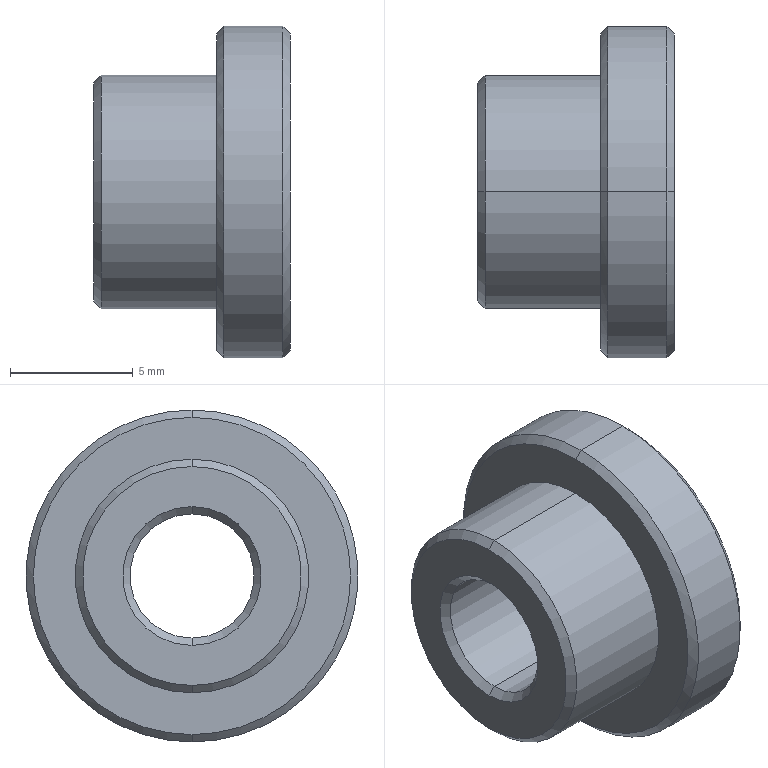Part | STEP file | Transition Guide Wheel | 1 solid | 19 faces | box 8 x 13.5 x 13.5 mm | volume 617.031 mm3 | cone 10 | cylinder 6 | plane 3 | commonest cylinder face diameters 5.05 x2 9.5 x2 13.5 x2
STEP:
#1=CARTESIAN_POINT('',(0.,0.,0.));
#2=DIRECTION('',(0.,0.,1.));
#3=DIRECTION('',(1.,0.,0.));
#4=AXIS2_PLACEMENT_3D('',#1,#2,#3);
#5=CARTESIAN_POINT('',(0.,0.,6.45));
#6=VERTEX_POINT('',#5);
#7=CARTESIAN_POINT('',(0.,0.,-6.45));
#8=VERTEX_POINT('',#7);
#9=CARTESIAN_POINT('',(0.,0.,0.));
#10=DIRECTION('',(-1.,0.,0.));
#11=DIRECTION('',(0.,0.,1.));
#12=AXIS2_PLACEMENT_3D('',#9,#10,#11);
#13=CIRCLE('',#12,6.45);
#14=CARTESIAN_POINT('',(0.3,0.,0.));
#15=DIRECTION('',(1.,0.,0.));
#16=DIRECTION('',(0.,0.,-1.));
#17=AXIS2_PLACEMENT_3D('',#14,#15,#16);
#18=CONICAL_SURFACE('',#17,6.75,0.7854);
#19=CARTESIAN_POINT('',(3.142,-0.3));
#20=DIRECTION('',(-1.,0.));
#21=VECTOR('',#20,1.);
#22=LINE('',#19,#21);
#23=(GEOMETRIC_REPRESENTATION_CONTEXT(2)PARAMETRIC_REPRESENTATION_CONTEXT()REPRESENTATION_CONTEXT('',''));
#24=DEFINITIONAL_REPRESENTATION('',(#22),#23);
#25=PCURVE('',#18,#24);
#26=CARTESIAN_POINT('',(0.,4.75,0.));
#27=DIRECTION('',(-1.,0.,0.));
#28=DIRECTION('',(0.,0.,1.));
#29=AXIS2_PLACEMENT_3D('',#26,#27,#28);
#30=PLANE('',#29);
#31=CARTESIAN_POINT('',(0.,-4.75));
#32=DIRECTION('',(1.,0.));
#33=AXIS2_PLACEMENT_2D('',#31,#32);
#34=CIRCLE('',#33,6.45);
#35=(GEOMETRIC_REPRESENTATION_CONTEXT(2)PARAMETRIC_REPRESENTATION_CONTEXT()REPRESENTATION_CONTEXT('',''));
#36=DEFINITIONAL_REPRESENTATION('',(#34),#35);
#37=PCURVE('',#30,#36);
#38=SURFACE_CURVE('',#13,(#25,#37),.PCURVE_S1.);
#39=EDGE_CURVE('',#6,#8,#38,.T.);
#40=ORIENTED_EDGE('',*,*,#39,.F.);
#41=CARTESIAN_POINT('',(0.3,0.,6.75));
#42=VERTEX_POINT('',#41);
#43=CARTESIAN_POINT('',(0.3,0.,6.75));
#44=DIRECTION('',(0.7071,0.,0.7071));
#45=VECTOR('',#44,1.);
#46=LINE('',#43,#45);
#47=CARTESIAN_POINT('',(3.142,0.));
#48=DIRECTION('',(0.,1.));
#49=VECTOR('',#48,1.);
#50=LINE('',#47,#49);
#51=(GEOMETRIC_REPRESENTATION_CONTEXT(2)PARAMETRIC_REPRESENTATION_CONTEXT()REPRESENTATION_CONTEXT('',''));
#52=DEFINITIONAL_REPRESENTATION('',(#50),#51);
#53=PCURVE('',#18,#52);
#54=CARTESIAN_POINT('',(0.3,0.,0.));
#55=DIRECTION('',(1.,0.,0.));
#56=DIRECTION('',(0.,0.,-1.));
#57=AXIS2_PLACEMENT_3D('',#54,#55,#56);
#58=CONICAL_SURFACE('',#57,6.75,0.7854);
#59=CARTESIAN_POINT('',(3.142,0.));
#60=DIRECTION('',(0.,1.));
#61=VECTOR('',#60,1.);
#62=LINE('',#59,#61);
#63=(GEOMETRIC_REPRESENTATION_CONTEXT(2)PARAMETRIC_REPRESENTATION_CONTEXT()REPRESENTATION_CONTEXT('',''));
#64=DEFINITIONAL_REPRESENTATION('',(#62),#63);
#65=PCURVE('',#58,#64);
#66=SURFACE_CURVE('',#46,(#53,#65),.PCURVE_S1.);
#67=EDGE_CURVE('',#6,#42,#66,.T.);
#68=ORIENTED_EDGE('',*,*,#67,.T.);
#69=CARTESIAN_POINT('',(0.3,0.,-6.75));
#70=VERTEX_POINT('',#69);
#71=CARTESIAN_POINT('',(0.3,0.,0.));
#72=DIRECTION('',(1.,0.,0.));
#73=DIRECTION('',(0.,0.,1.));
#74=AXIS2_PLACEMENT_3D('',#71,#72,#73);
#75=CIRCLE('',#74,6.75);
#76=CARTESIAN_POINT('',(-3.142,0.));
#77=DIRECTION('',(1.,0.));
#78=VECTOR('',#77,1.);
#79=LINE('',#76,#78);
#80=(GEOMETRIC_REPRESENTATION_CONTEXT(2)PARAMETRIC_REPRESENTATION_CONTEXT()REPRESENTATION_CONTEXT('',''));
#81=DEFINITIONAL_REPRESENTATION('',(#79),#80);
#82=PCURVE('',#18,#81);
#83=CARTESIAN_POINT('',(0.,0.,0.));
#84=DIRECTION('',(1.,0.,0.));
#85=DIRECTION('',(0.,0.,-1.));
#86=AXIS2_PLACEMENT_3D('',#83,#84,#85);
#87=CYLINDRICAL_SURFACE('',#86,6.75);
#88=CARTESIAN_POINT('',(-3.142,0.3));
#89=DIRECTION('',(1.,0.));
#90=VECTOR('',#89,1.);
#91=LINE('',#88,#90);
#92=(GEOMETRIC_REPRESENTATION_CONTEXT(2)PARAMETRIC_REPRESENTATION_CONTEXT()REPRESENTATION_CONTEXT('',''));
#93=DEFINITIONAL_REPRESENTATION('',(#91),#92);
#94=PCURVE('',#87,#93);
#95=SURFACE_CURVE('',#75,(#82,#94),.PCURVE_S1.);
#96=EDGE_CURVE('',#70,#42,#95,.T.);
#97=ORIENTED_EDGE('',*,*,#96,.F.);
#98=CARTESIAN_POINT('',(0.3,0.,-6.75));
#99=DIRECTION('',(0.7071,0.,-0.7071));
#100=VECTOR('',#99,1.);
#101=LINE('',#98,#100);
#102=CARTESIAN_POINT('',(0.,0.));
#103=DIRECTION('',(0.,1.));
#104=VECTOR('',#103,1.);
#105=LINE('',#102,#104);
#106=(GEOMETRIC_REPRESENTATION_CONTEXT(2)PARAMETRIC_REPRESENTATION_CONTEXT()REPRESENTATION_CONTEXT('',''));
#107=DEFINITIONAL_REPRESENTATION('',(#105),#106);
#108=PCURVE('',#18,#107);
#109=CARTESIAN_POINT('',(6.283,0.));
#110=DIRECTION('',(0.,1.));
#111=VECTOR('',#110,1.);
#112=LINE('',#109,#111);
#113=(GEOMETRIC_REPRESENTATION_CONTEXT(2)PARAMETRIC_REPRESENTATION_CONTEXT()REPRESENTATION_CONTEXT('',''));
#114=DEFINITIONAL_REPRESENTATION('',(#112),#113);
#115=PCURVE('',#58,#114);
#116=SURFACE_CURVE('',#101,(#108,#115),.PCURVE_S1.);
#117=EDGE_CURVE('',#8,#70,#116,.T.);
#118=ORIENTED_EDGE('',*,*,#117,.F.);
#119=EDGE_LOOP('',(#40,#68,#97,#118));
#120=FACE_BOUND('',#119,.T.);
#121=ADVANCED_FACE('',(#120),#18,.T.);
#122=CARTESIAN_POINT('',(3.,0.,-6.45));
#123=VERTEX_POINT('',#122);
#124=CARTESIAN_POINT('',(3.,0.,6.45));
#125=VERTEX_POINT('',#124);
#126=CARTESIAN_POINT('',(3.,0.,0.));
#127=DIRECTION('',(1.,0.,0.));
#128=DIRECTION('',(0.,0.,-1.));
#129=AXIS2_PLACEMENT_3D('',#126,#127,#128);
#130=CIRCLE('',#129,6.45);
#131=CARTESIAN_POINT('',(3.,0.,0.));
#132=DIRECTION('',(-1.,0.,0.));
#133=DIRECTION('',(0.,0.,1.));
#134=AXIS2_PLACEMENT_3D('',#131,#132,#133);
#135=CONICAL_SURFACE('',#134,6.45,0.7854);
#136=CARTESIAN_POINT('',(3.142,0.));
#137=DIRECTION('',(-1.,0.));
#138=VECTOR('',#137,1.);
#139=LINE('',#136,#138);
#140=(GEOMETRIC_REPRESENTATION_CONTEXT(2)PARAMETRIC_REPRESENTATION_CONTEXT()REPRESENTATION_CONTEXT('',''));
#141=DEFINITIONAL_REPRESENTATION('',(#139),#140);
#142=PCURVE('',#135,#141);
#143=CARTESIAN_POINT('',(3.,6.75,0.));
#144=DIRECTION('',(1.,0.,0.));
#145=DIRECTION('',(0.,0.,-1.));
#146=AXIS2_PLACEMENT_3D('',#143,#144,#145);
#147=PLANE('',#146);
#148=CARTESIAN_POINT('',(0.,-6.75));
#149=DIRECTION('',(1.,0.));
#150=AXIS2_PLACEMENT_2D('',#148,#149);
#151=CIRCLE('',#150,6.45);
#152=(GEOMETRIC_REPRESENTATION_CONTEXT(2)PARAMETRIC_REPRESENTATION_CONTEXT()REPRESENTATION_CONTEXT('',''));
#153=DEFINITIONAL_REPRESENTATION('',(#151),#152);
#154=PCURVE('',#147,#153);
#155=SURFACE_CURVE('',#130,(#142,#154),.PCURVE_S1.);
#156=EDGE_CURVE('',#123,#125,#155,.T.);
#157=ORIENTED_EDGE('',*,*,#156,.F.);
#158=CARTESIAN_POINT('',(2.7,0.,-6.75));
#159=VERTEX_POINT('',#158);
#160=CARTESIAN_POINT('',(3.,0.,-6.45));
#161=DIRECTION('',(-0.7071,0.,-0.7071));
#162=VECTOR('',#161,1.);
#163=LINE('',#160,#162);
#164=CARTESIAN_POINT('',(3.142,0.));
#165=DIRECTION('',(0.,1.));
#166=VECTOR('',#165,1.);
#167=LINE('',#164,#166);
#168=(GEOMETRIC_REPRESENTATION_CONTEXT(2)PARAMETRIC_REPRESENTATION_CONTEXT()REPRESENTATION_CONTEXT('',''));
#169=DEFINITIONAL_REPRESENTATION('',(#167),#168);
#170=PCURVE('',#135,#169);
#171=CARTESIAN_POINT('',(3.,0.,0.));
#172=DIRECTION('',(-1.,0.,0.));
#173=DIRECTION('',(0.,0.,1.));
#174=AXIS2_PLACEMENT_3D('',#171,#172,#173);
#175=CONICAL_SURFACE('',#174,6.45,0.7854);
#176=CARTESIAN_POINT('',(3.142,0.));
#177=DIRECTION('',(0.,1.));
#178=VECTOR('',#177,1.);
#179=LINE('',#176,#178);
#180=(GEOMETRIC_REPRESENTATION_CONTEXT(2)PARAMETRIC_REPRESENTATION_CONTEXT()REPRESENTATION_CONTEXT('',''));
#181=DEFINITIONAL_REPRESENTATION('',(#179),#180);
#182=PCURVE('',#175,#181);
#183=SURFACE_CURVE('',#163,(#170,#182),.PCURVE_S1.);
#184=EDGE_CURVE('',#123,#159,#183,.T.);
#185=ORIENTED_EDGE('',*,*,#184,.T.);
#186=CARTESIAN_POINT('',(2.7,0.,6.75));
#187=VERTEX_POINT('',#186);
#188=CARTESIAN_POINT('',(2.7,0.,0.));
#189=DIRECTION('',(-1.,0.,0.));
#190=DIRECTION('',(0.,0.,-1.));
#191=AXIS2_PLACEMENT_3D('',#188,#189,#190);
#192=CIRCLE('',#191,6.75);
#193=CARTESIAN_POINT('',(-3.142,0.3));
#194=DIRECTION('',(1.,0.));
#195=VECTOR('',#194,1.);
#196=LINE('',#193,#195);
#197=(GEOMETRIC_REPRESENTATION_CONTEXT(2)PARAMETRIC_REPRESENTATION_CONTEXT()REPRESENTATION_CONTEXT('',''));
#198=DEFINITIONAL_REPRESENTATION('',(#196),#197);
#199=PCURVE('',#135,#198);
#200=CARTESIAN_POINT('',(6.283,2.7));
#201=DIRECTION('',(-1.,0.));
#202=VECTOR('',#201,1.);
#203=LINE('',#200,#202);
#204=(GEOMETRIC_REPRESENTATION_CONTEXT(2)PARAMETRIC_REPRESENTATION_CONTEXT()REPRESENTATION_CONTEXT('',''));
#205=DEFINITIONAL_REPRESENTATION('',(#203),#204);
#206=PCURVE('',#87,#205);
#207=SURFACE_CURVE('',#192,(#199,#206),.PCURVE_S1.);
#208=EDGE_CURVE('',#187,#159,#207,.T.);
#209=ORIENTED_EDGE('',*,*,#208,.F.);
#210=CARTESIAN_POINT('',(3.,0.,6.45));
#211=DIRECTION('',(-0.7071,0.,0.7071));
#212=VECTOR('',#211,1.);
#213=LINE('',#210,#212);
#214=CARTESIAN_POINT('',(0.,0.));
#215=DIRECTION('',(0.,1.));
#216=VECTOR('',#215,1.);
#217=LINE('',#214,#216);
#218=(GEOMETRIC_REPRESENTATION_CONTEXT(2)PARAMETRIC_REPRESENTATION_CONTEXT()REPRESENTATION_CONTEXT('',''));
#219=DEFINITIONAL_REPRESENTATION('',(#217),#218);
#220=PCURVE('',#135,#219);
#221=CARTESIAN_POINT('',(6.283,0.));
#222=DIRECTION('',(0.,1.));
#223=VECTOR('',#222,1.);
#224=LINE('',#221,#223);
#225=(GEOMETRIC_REPRESENTATION_CONTEXT(2)PARAMETRIC_REPRESENTATION_CONTEXT()REPRESENTATION_CONTEXT('',''));
#226=DEFINITIONAL_REPRESENTATION('',(#224),#225);
#227=PCURVE('',#175,#226);
#228=SURFACE_CURVE('',#213,(#220,#227),.PCURVE_S1.);
#229=EDGE_CURVE('',#125,#187,#228,.T.);
#230=ORIENTED_EDGE('',*,*,#229,.F.);
#231=EDGE_LOOP('',(#157,#185,#209,#230));
#232=FACE_BOUND('',#231,.T.);
#233=ADVANCED_FACE('',(#232),#135,.T.);
#234=CARTESIAN_POINT('',(2.7,0.,-2.525));
#235=VERTEX_POINT('',#234);
#236=CARTESIAN_POINT('',(3.,0.,-2.825));
#237=VERTEX_POINT('',#236);
#238=CARTESIAN_POINT('',(2.7,0.,-2.525));
#239=DIRECTION('',(0.7071,0.,-0.7071));
#240=VECTOR('',#239,1.);
#241=LINE('',#238,#240);
#242=CARTESIAN_POINT('',(2.7,0.,0.));
#243=DIRECTION('',(1.,0.,0.));
#244=DIRECTION('',(0.,0.,-1.));
#245=AXIS2_PLACEMENT_3D('',#242,#243,#244);
#246=CONICAL_SURFACE('',#245,2.525,0.7854);
#247=CARTESIAN_POINT('',(6.283,0.));
#248=DIRECTION('',(0.,1.));
#249=VECTOR('',#248,1.);
#250=LINE('',#247,#249);
#251=(GEOMETRIC_REPRESENTATION_CONTEXT(2)PARAMETRIC_REPRESENTATION_CONTEXT()REPRESENTATION_CONTEXT('',''));
#252=DEFINITIONAL_REPRESENTATION('',(#250),#251);
#253=PCURVE('',#246,#252);
#254=CARTESIAN_POINT('',(2.7,0.,0.));
#255=DIRECTION('',(1.,0.,0.));
#256=DIRECTION('',(0.,0.,-1.));
#257=AXIS2_PLACEMENT_3D('',#254,#255,#256);
#258=CONICAL_SURFACE('',#257,2.525,0.7854);
#259=CARTESIAN_POINT('',(0.,0.));
#260=DIRECTION('',(0.,1.));
#261=VECTOR('',#260,1.);
#262=LINE('',#259,#261);
#263=(GEOMETRIC_REPRESENTATION_CONTEXT(2)PARAMETRIC_REPRESENTATION_CONTEXT()REPRESENTATION_CONTEXT('',''));
#264=DEFINITIONAL_REPRESENTATION('',(#262),#263);
#265=PCURVE('',#258,#264);
#266=SURFACE_CURVE('',#241,(#253,#265),.PCURVE_S1.);
#267=EDGE_CURVE('',#235,#237,#266,.T.);
#268=ORIENTED_EDGE('',*,*,#267,.T.);
#269=CARTESIAN_POINT('',(3.,0.,2.825));
#270=VERTEX_POINT('',#269);
#271=CARTESIAN_POINT('',(3.,0.,0.));
#272=DIRECTION('',(-1.,0.,0.));
#273=DIRECTION('',(0.,0.,-1.));
#274=AXIS2_PLACEMENT_3D('',#271,#272,#273);
#275=CIRCLE('',#274,2.825);
#276=CARTESIAN_POINT('',(6.283,0.3));
#277=DIRECTION('',(-1.,0.));
#278=VECTOR('',#277,1.);
#279=LINE('',#276,#278);
#280=(GEOMETRIC_REPRESENTATION_CONTEXT(2)PARAMETRIC_REPRESENTATION_CONTEXT()REPRESENTATION_CONTEXT('',''));
#281=DEFINITIONAL_REPRESENTATION('',(#279),#280);
#282=PCURVE('',#246,#281);
#283=CARTESIAN_POINT('',(2.825,-6.75));
#284=CARTESIAN_POINT('',(2.825,-11.643));
#285=CARTESIAN_POINT('',(-1.413,-9.197));
#286=CARTESIAN_POINT('',(-5.65,-6.75));
#287=CARTESIAN_POINT('',(-1.413,-4.303));
#288=CARTESIAN_POINT('',(2.825,-1.857));
#289=CARTESIAN_POINT('',(2.825,-6.75));
#290=(BOUNDED_CURVE()B_SPLINE_CURVE(2,(#283,#284,#285,#286,#287,#288,#289),.UNSPECIFIED.,.T.,.F.)B_SPLINE_CURVE_WITH_KNOTS((1,2,2,2,2,1),(-2.094,0.,2.094,4.189,6.283,8.378),.UNSPECIFIED.)CURVE()GEOMETRIC_REPRESENTATION_ITEM()RATIONAL_B_SPLINE_CURVE((1.,0.5,1.,0.5,1.,0.5,1.))REPRESENTATION_ITEM(''));
#291=(GEOMETRIC_REPRESENTATION_CONTEXT(2)PARAMETRIC_REPRESENTATION_CONTEXT()REPRESENTATION_CONTEXT('',''));
#292=DEFINITIONAL_REPRESENTATION('',(#290),#291);
#293=PCURVE('',#147,#292);
#294=SURFACE_CURVE('',#275,(#282,#293),.PCURVE_S1.);
#295=EDGE_CURVE('',#237,#270,#294,.T.);
#296=ORIENTED_EDGE('',*,*,#295,.T.);
#297=CARTESIAN_POINT('',(2.7,0.,2.525));
#298=VERTEX_POINT('',#297);
#299=CARTESIAN_POINT('',(2.7,0.,2.525));
#300=DIRECTION('',(0.7071,0.,0.7071));
#301=VECTOR('',#300,1.);
#302=LINE('',#299,#301);
#303=CARTESIAN_POINT('',(3.142,0.));
#304=DIRECTION('',(0.,1.));
#305=VECTOR('',#304,1.);
#306=LINE('',#303,#305);
#307=(GEOMETRIC_REPRESENTATION_CONTEXT(2)PARAMETRIC_REPRESENTATION_CONTEXT()REPRESENTATION_CONTEXT('',''));
#308=DEFINITIONAL_REPRESENTATION('',(#306),#307);
#309=PCURVE('',#246,#308);
#310=CARTESIAN_POINT('',(3.142,0.));
#311=DIRECTION('',(0.,1.));
#312=VECTOR('',#311,1.);
#313=LINE('',#310,#312);
#314=(GEOMETRIC_REPRESENTATION_CONTEXT(2)PARAMETRIC_REPRESENTATION_CONTEXT()REPRESENTATION_CONTEXT('',''));
#315=DEFINITIONAL_REPRESENTATION('',(#313),#314);
#316=PCURVE('',#258,#315);
#317=SURFACE_CURVE('',#302,(#309,#316),.PCURVE_S1.);
#318=EDGE_CURVE('',#298,#270,#317,.T.);
#319=ORIENTED_EDGE('',*,*,#318,.F.);
#320=CARTESIAN_POINT('',(2.7,0.,0.));
#321=DIRECTION('',(1.,0.,0.));
#322=DIRECTION('',(0.,0.,-1.));
#323=AXIS2_PLACEMENT_3D('',#320,#321,#322);
#324=CIRCLE('',#323,2.525);
#325=CARTESIAN_POINT('',(0.,0.));
#326=DIRECTION('',(1.,0.));
#327=VECTOR('',#326,1.);
#328=LINE('',#325,#327);
#329=(GEOMETRIC_REPRESENTATION_CONTEXT(2)PARAMETRIC_REPRESENTATION_CONTEXT()REPRESENTATION_CONTEXT('',''));
#330=DEFINITIONAL_REPRESENTATION('',(#328),#329);
#331=PCURVE('',#246,#330);
#332=CARTESIAN_POINT('',(0.,0.,0.));
#333=DIRECTION('',(1.,0.,0.));
#334=DIRECTION('',(0.,0.,-1.));
#335=AXIS2_PLACEMENT_3D('',#332,#333,#334);
#336=CYLINDRICAL_SURFACE('',#335,2.525);
#337=CARTESIAN_POINT('',(0.,2.7));
#338=DIRECTION('',(1.,0.));
#339=VECTOR('',#338,1.);
#340=LINE('',#337,#339);
#341=(GEOMETRIC_REPRESENTATION_CONTEXT(2)PARAMETRIC_REPRESENTATION_CONTEXT()REPRESENTATION_CONTEXT('',''));
#342=DEFINITIONAL_REPRESENTATION('',(#340),#341);
#343=PCURVE('',#336,#342);
#344=SURFACE_CURVE('',#324,(#331,#343),.PCURVE_S1.);
#345=EDGE_CURVE('',#298,#235,#344,.T.);
#346=ORIENTED_EDGE('',*,*,#345,.T.);
#347=EDGE_LOOP('',(#268,#296,#319,#346));
#348=FACE_BOUND('',#347,.F.);
#349=ADVANCED_FACE('',(#348),#246,.F.);
#350=CARTESIAN_POINT('',(-4.7,0.,2.525));
#351=VERTEX_POINT('',#350);
#352=CARTESIAN_POINT('',(-5.,0.,2.825));
#353=VERTEX_POINT('',#352);
#354=CARTESIAN_POINT('',(-5.,0.,2.825));
#355=DIRECTION('',(-0.7071,0.,0.7071));
#356=VECTOR('',#355,1.);
#357=LINE('',#354,#356);
#358=CARTESIAN_POINT('',(-5.,0.,0.));
#359=DIRECTION('',(-1.,0.,0.));
#360=DIRECTION('',(0.,0.,1.));
#361=AXIS2_PLACEMENT_3D('',#358,#359,#360);
#362=CONICAL_SURFACE('',#361,2.825,0.7854);
#363=CARTESIAN_POINT('',(6.283,0.));
#364=DIRECTION('',(0.,1.));
#365=VECTOR('',#364,1.);
#366=LINE('',#363,#365);
#367=(GEOMETRIC_REPRESENTATION_CONTEXT(2)PARAMETRIC_REPRESENTATION_CONTEXT()REPRESENTATION_CONTEXT('',''));
#368=DEFINITIONAL_REPRESENTATION('',(#366),#367);
#369=PCURVE('',#362,#368);
#370=CARTESIAN_POINT('',(-5.,0.,0.));
#371=DIRECTION('',(-1.,0.,0.));
#372=DIRECTION('',(0.,0.,1.));
#373=AXIS2_PLACEMENT_3D('',#370,#371,#372);
#374=CONICAL_SURFACE('',#373,2.825,0.7854);
#375=CARTESIAN_POINT('',(0.,0.));
#376=DIRECTION('',(0.,1.));
#377=VECTOR('',#376,1.);
#378=LINE('',#375,#377);
#379=(GEOMETRIC_REPRESENTATION_CONTEXT(2)PARAMETRIC_REPRESENTATION_CONTEXT()REPRESENTATION_CONTEXT('',''));
#380=DEFINITIONAL_REPRESENTATION('',(#378),#379);
#381=PCURVE('',#374,#380);
#382=SURFACE_CURVE('',#357,(#369,#381),.PCURVE_S1.);
#383=EDGE_CURVE('',#351,#353,#382,.T.);
#384=ORIENTED_EDGE('',*,*,#383,.T.);
#385=CARTESIAN_POINT('',(-5.,0.,-2.825));
#386=VERTEX_POINT('',#385);
#387=CARTESIAN_POINT('',(-5.,0.,0.));
#388=DIRECTION('',(1.,0.,0.));
#389=DIRECTION('',(0.,0.,1.));
#390=AXIS2_PLACEMENT_3D('',#387,#388,#389);
#391=CIRCLE('',#390,2.825);
#392=CARTESIAN_POINT('',(6.283,0.));
#393=DIRECTION('',(-1.,0.));
#394=VECTOR('',#393,1.);
#395=LINE('',#392,#394);
#396=(GEOMETRIC_REPRESENTATION_CONTEXT(2)PARAMETRIC_REPRESENTATION_CONTEXT()REPRESENTATION_CONTEXT('',''));
#397=DEFINITIONAL_REPRESENTATION('',(#395),#396);
#398=PCURVE('',#362,#397);
#399=CARTESIAN_POINT('',(-5.,2.525,0.));
#400=DIRECTION('',(-1.,0.,0.));
#401=DIRECTION('',(0.,0.,1.));
#402=AXIS2_PLACEMENT_3D('',#399,#400,#401);
#403=PLANE('',#402);
#404=CARTESIAN_POINT('',(2.825,-2.525));
#405=CARTESIAN_POINT('',(2.825,-7.418));
#406=CARTESIAN_POINT('',(-1.413,-4.972));
#407=CARTESIAN_POINT('',(-5.65,-2.525));
#408=CARTESIAN_POINT('',(-1.413,-0.07848));
#409=CARTESIAN_POINT('',(2.825,2.368));
#410=CARTESIAN_POINT('',(2.825,-2.525));
#411=(BOUNDED_CURVE()B_SPLINE_CURVE(2,(#404,#405,#406,#407,#408,#409,#410),.UNSPECIFIED.,.T.,.F.)B_SPLINE_CURVE_WITH_KNOTS((1,2,2,2,2,1),(-2.094,0.,2.094,4.189,6.283,8.378),.UNSPECIFIED.)CURVE()GEOMETRIC_REPRESENTATION_ITEM()RATIONAL_B_SPLINE_CURVE((1.,0.5,1.,0.5,1.,0.5,1.))REPRESENTATION_ITEM(''));
#412=(GEOMETRIC_REPRESENTATION_CONTEXT(2)PARAMETRIC_REPRESENTATION_CONTEXT()REPRESENTATION_CONTEXT('',''));
#413=DEFINITIONAL_REPRESENTATION('',(#411),#412);
#414=PCURVE('',#403,#413);
#415=SURFACE_CURVE('',#391,(#398,#414),.PCURVE_S1.);
#416=EDGE_CURVE('',#353,#386,#415,.T.);
#417=ORIENTED_EDGE('',*,*,#416,.T.);
#418=CARTESIAN_POINT('',(-4.7,0.,-2.525));
#419=VERTEX_POINT('',#418);
#420=CARTESIAN_POINT('',(-5.,0.,-2.825));
#421=DIRECTION('',(-0.7071,0.,-0.7071));
#422=VECTOR('',#421,1.);
#423=LINE('',#420,#422);
#424=CARTESIAN_POINT('',(3.142,0.));
#425=DIRECTION('',(0.,1.));
#426=VECTOR('',#425,1.);
#427=LINE('',#424,#426);
#428=(GEOMETRIC_REPRESENTATION_CONTEXT(2)PARAMETRIC_REPRESENTATION_CONTEXT()REPRESENTATION_CONTEXT('',''));
#429=DEFINITIONAL_REPRESENTATION('',(#427),#428);
#430=PCURVE('',#362,#429);
#431=CARTESIAN_POINT('',(3.142,0.));
#432=DIRECTION('',(0.,1.));
#433=VECTOR('',#432,1.);
#434=LINE('',#431,#433);
#435=(GEOMETRIC_REPRESENTATION_CONTEXT(2)PARAMETRIC_REPRESENTATION_CONTEXT()REPRESENTATION_CONTEXT('',''));
#436=DEFINITIONAL_REPRESENTATION('',(#434),#435);
#437=PCURVE('',#374,#436);
#438=SURFACE_CURVE('',#423,(#430,#437),.PCURVE_S1.);
#439=EDGE_CURVE('',#419,#386,#438,.T.);
#440=ORIENTED_EDGE('',*,*,#439,.F.);
#441=CARTESIAN_POINT('',(-4.7,0.,0.));
#442=DIRECTION('',(-1.,0.,0.));
#443=DIRECTION('',(0.,0.,1.));
#444=AXIS2_PLACEMENT_3D('',#441,#442,#443);
#445=CIRCLE('',#444,2.525);
#446=CARTESIAN_POINT('',(0.,-0.3));
#447=DIRECTION('',(1.,0.));
#448=VECTOR('',#447,1.);
#449=LINE('',#446,#448);
#450=(GEOMETRIC_REPRESENTATION_CONTEXT(2)PARAMETRIC_REPRESENTATION_CONTEXT()REPRESENTATION_CONTEXT('',''));
#451=DEFINITIONAL_REPRESENTATION('',(#449),#450);
#452=PCURVE('',#362,#451);
#453=CARTESIAN_POINT('',(9.425,-4.7));
#454=DIRECTION('',(-1.,0.));
#455=VECTOR('',#454,1.);
#456=LINE('',#453,#455);
#457=(GEOMETRIC_REPRESENTATION_CONTEXT(2)PARAMETRIC_REPRESENTATION_CONTEXT()REPRESENTATION_CONTEXT('',''));
#458=DEFINITIONAL_REPRESENTATION('',(#456),#457);
#459=PCURVE('',#336,#458);
#460=SURFACE_CURVE('',#445,(#452,#459),.PCURVE_S1.);
#461=EDGE_CURVE('',#419,#351,#460,.T.);
#462=ORIENTED_EDGE('',*,*,#461,.T.);
#463=EDGE_LOOP('',(#384,#417,#440,#462));
#464=FACE_BOUND('',#463,.F.);
#465=ADVANCED_FACE('',(#464),#362,.F.);
#466=CARTESIAN_POINT('',(-5.,0.,4.45));
#467=VERTEX_POINT('',#466);
#468=CARTESIAN_POINT('',(-5.,0.,-4.45));
#469=VERTEX_POINT('',#468);
#470=CARTESIAN_POINT('',(-5.,0.,0.));
#471=DIRECTION('',(-1.,0.,0.));
#472=DIRECTION('',(0.,0.,1.));
#473=AXIS2_PLACEMENT_3D('',#470,#471,#472);
#474=CIRCLE('',#473,4.45);
#475=CARTESIAN_POINT('',(-4.7,0.,0.));
#476=DIRECTION('',(1.,0.,0.));
#477=DIRECTION('',(0.,0.,-1.));
#478=AXIS2_PLACEMENT_3D('',#475,#476,#477);
#479=CONICAL_SURFACE('',#478,4.75,0.7854);
#480=CARTESIAN_POINT('',(3.142,-0.3));
#481=DIRECTION('',(-1.,0.));
#482=VECTOR('',#481,1.);
#483=LINE('',#480,#482);
#484=(GEOMETRIC_REPRESENTATION_CONTEXT(2)PARAMETRIC_REPRESENTATION_CONTEXT()REPRESENTATION_CONTEXT('',''));
#485=DEFINITIONAL_REPRESENTATION('',(#483),#484);
#486=PCURVE('',#479,#485);
#487=CARTESIAN_POINT('',(0.,-2.525));
#488=DIRECTION('',(1.,0.));
#489=AXIS2_PLACEMENT_2D('',#487,#488);
#490=CIRCLE('',#489,4.45);
#491=(GEOMETRIC_REPRESENTATION_CONTEXT(2)PARAMETRIC_REPRESENTATION_CONTEXT()REPRESENTATION_CONTEXT('',''));
#492=DEFINITIONAL_REPRESENTATION('',(#490),#491);
#493=PCURVE('',#403,#492);
#494=SURFACE_CURVE('',#474,(#486,#493),.PCURVE_S1.);
#495=EDGE_CURVE('',#467,#469,#494,.T.);
#496=ORIENTED_EDGE('',*,*,#495,.F.);
#497=CARTESIAN_POINT('',(-4.7,0.,4.75));
#498=VERTEX_POINT('',#497);
#499=CARTESIAN_POINT('',(-4.7,0.,4.75));
#500=DIRECTION('',(0.7071,0.,0.7071));
#501=VECTOR('',#500,1.);
#502=LINE('',#499,#501);
#503=CARTESIAN_POINT('',(3.142,0.));
#504=DIRECTION('',(0.,1.));
#505=VECTOR('',#504,1.);
#506=LINE('',#503,#505);
#507=(GEOMETRIC_REPRESENTATION_CONTEXT(2)PARAMETRIC_REPRESENTATION_CONTEXT()REPRESENTATION_CONTEXT('',''));
#508=DEFINITIONAL_REPRESENTATION('',(#506),#507);
#509=PCURVE('',#479,#508);
#510=CARTESIAN_POINT('',(-4.7,0.,0.));
#511=DIRECTION('',(1.,0.,0.));
#512=DIRECTION('',(0.,0.,-1.));
#513=AXIS2_PLACEMENT_3D('',#510,#511,#512);
#514=CONICAL_SURFACE('',#513,4.75,0.7854);
#515=CARTESIAN_POINT('',(3.142,0.));
#516=DIRECTION('',(0.,1.));
#517=VECTOR('',#516,1.);
#518=LINE('',#515,#517);
#519=(GEOMETRIC_REPRESENTATION_CONTEXT(2)PARAMETRIC_REPRESENTATION_CONTEXT()REPRESENTATION_CONTEXT('',''));
#520=DEFINITIONAL_REPRESENTATION('',(#518),#519);
#521=PCURVE('',#514,#520);
#522=SURFACE_CURVE('',#502,(#509,#521),.PCURVE_S1.);
#523=EDGE_CURVE('',#467,#498,#522,.T.);
#524=ORIENTED_EDGE('',*,*,#523,.T.);
#525=CARTESIAN_POINT('',(-4.7,0.,-4.75));
#526=VERTEX_POINT('',#525);
#527=CARTESIAN_POINT('',(-4.7,0.,0.));
#528=DIRECTION('',(1.,0.,0.));
#529=DIRECTION('',(0.,0.,1.));
#530=AXIS2_PLACEMENT_3D('',#527,#528,#529);
#531=CIRCLE('',#530,4.75);
#532=CARTESIAN_POINT('',(-3.142,0.));
#533=DIRECTION('',(1.,0.));
#534=VECTOR('',#533,1.);
#535=LINE('',#532,#534);
#536=(GEOMETRIC_REPRESENTATION_CONTEXT(2)PARAMETRIC_REPRESENTATION_CONTEXT()REPRESENTATION_CONTEXT('',''));
#537=DEFINITIONAL_REPRESENTATION('',(#535),#536);
#538=PCURVE('',#479,#537);
#539=CARTESIAN_POINT('',(0.,0.,0.));
#540=DIRECTION('',(1.,0.,0.));
#541=DIRECTION('',(0.,0.,-1.));
#542=AXIS2_PLACEMENT_3D('',#539,#540,#541);
#543=CYLINDRICAL_SURFACE('',#542,4.75);
#544=CARTESIAN_POINT('',(-3.142,-4.7));
#545=DIRECTION('',(1.,0.));
#546=VECTOR('',#545,1.);
#547=LINE('',#544,#546);
#548=(GEOMETRIC_REPRESENTATION_CONTEXT(2)PARAMETRIC_REPRESENTATION_CONTEXT()REPRESENTATION_CONTEXT('',''));
#549=DEFINITIONAL_REPRESENTATION('',(#547),#548);
#550=PCURVE('',#543,#549);
#551=SURFACE_CURVE('',#531,(#538,#550),.PCURVE_S1.);
#552=EDGE_CURVE('',#526,#498,#551,.T.);
#553=ORIENTED_EDGE('',*,*,#552,.F.);
#554=CARTESIAN_POINT('',(-4.7,0.,-4.75));
#555=DIRECTION('',(0.7071,0.,-0.7071));
#556=VECTOR('',#555,1.);
#557=LINE('',#554,#556);
#558=CARTESIAN_POINT('',(0.,0.));
#559=DIRECTION('',(0.,1.));
#560=VECTOR('',#559,1.);
#561=LINE('',#558,#560);
#562=(GEOMETRIC_REPRESENTATION_CONTEXT(2)PARAMETRIC_REPRESENTATION_CONTEXT()REPRESENTATION_CONTEXT('',''));
#563=DEFINITIONAL_REPRESENTATION('',(#561),#562);
#564=PCURVE('',#479,#563);
#565=CARTESIAN_POINT('',(6.283,0.));
#566=DIRECTION('',(0.,1.));
#567=VECTOR('',#566,1.);
#568=LINE('',#565,#567);
#569=(GEOMETRIC_REPRESENTATION_CONTEXT(2)PARAMETRIC_REPRESENTATION_CONTEXT()REPRESENTATION_CONTEXT('',''));
#570=DEFINITIONAL_REPRESENTATION('',(#568),#569);
#571=PCURVE('',#514,#570);
#572=SURFACE_CURVE('',#557,(#564,#571),.PCURVE_S1.);
#573=EDGE_CURVE('',#469,#526,#572,.T.);
#574=ORIENTED_EDGE('',*,*,#573,.F.);
#575=EDGE_LOOP('',(#496,#524,#553,#574));
#576=FACE_BOUND('',#575,.T.);
#577=ADVANCED_FACE('',(#576),#479,.T.);
#578=ORIENTED_EDGE('',*,*,#96,.T.);
#579=CARTESIAN_POINT('',(0.,0.,6.75));
#580=DIRECTION('',(1.,0.,0.));
#581=VECTOR('',#580,1.);
#582=LINE('',#579,#581);
#583=CARTESIAN_POINT('',(3.142,0.));
#584=DIRECTION('',(0.,1.));
#585=VECTOR('',#584,1.);
#586=LINE('',#583,#585);
#587=(GEOMETRIC_REPRESENTATION_CONTEXT(2)PARAMETRIC_REPRESENTATION_CONTEXT()REPRESENTATION_CONTEXT('',''));
#588=DEFINITIONAL_REPRESENTATION('',(#586),#587);
#589=PCURVE('',#87,#588);
#590=CARTESIAN_POINT('',(0.,0.,0.));
#591=DIRECTION('',(1.,0.,0.));
#592=DIRECTION('',(0.,0.,-1.));
#593=AXIS2_PLACEMENT_3D('',#590,#591,#592);
#594=CYLINDRICAL_SURFACE('',#593,6.75);
#595=CARTESIAN_POINT('',(3.142,0.));
#596=DIRECTION('',(0.,1.));
#597=VECTOR('',#596,1.);
#598=LINE('',#595,#597);
#599=(GEOMETRIC_REPRESENTATION_CONTEXT(2)PARAMETRIC_REPRESENTATION_CONTEXT()REPRESENTATION_CONTEXT('',''));
#600=DEFINITIONAL_REPRESENTATION('',(#598),#599);
#601=PCURVE('',#594,#600);
#602=SURFACE_CURVE('',#582,(#589,#601),.PCURVE_S1.);
#603=EDGE_CURVE('',#42,#187,#602,.T.);
#604=ORIENTED_EDGE('',*,*,#603,.T.);
#605=ORIENTED_EDGE('',*,*,#208,.T.);
#606=CARTESIAN_POINT('',(0.,0.,-6.75));
#607=DIRECTION('',(1.,0.,0.));
#608=VECTOR('',#607,1.);
#609=LINE('',#606,#608);
#610=CARTESIAN_POINT('',(0.,0.));
#611=DIRECTION('',(0.,1.));
#612=VECTOR('',#611,1.);
#613=LINE('',#610,#612);
#614=(GEOMETRIC_REPRESENTATION_CONTEXT(2)PARAMETRIC_REPRESENTATION_CONTEXT()REPRESENTATION_CONTEXT('',''));
#615=DEFINITIONAL_REPRESENTATION('',(#613),#614);
#616=PCURVE('',#87,#615);
#617=CARTESIAN_POINT('',(6.283,0.));
#618=DIRECTION('',(0.,1.));
#619=VECTOR('',#618,1.);
#620=LINE('',#617,#619);
#621=(GEOMETRIC_REPRESENTATION_CONTEXT(2)PARAMETRIC_REPRESENTATION_CONTEXT()REPRESENTATION_CONTEXT('',''));
#622=DEFINITIONAL_REPRESENTATION('',(#620),#621);
#623=PCURVE('',#594,#622);
#624=SURFACE_CURVE('',#609,(#616,#623),.PCURVE_S1.);
#625=EDGE_CURVE('',#70,#159,#624,.T.);
#626=ORIENTED_EDGE('',*,*,#625,.F.);
#627=EDGE_LOOP('',(#578,#604,#605,#626));
#628=FACE_BOUND('',#627,.T.);
#629=ADVANCED_FACE('',(#628),#87,.T.);
#630=ORIENTED_EDGE('',*,*,#552,.T.);
#631=CARTESIAN_POINT('',(0.,0.,4.75));
#632=VERTEX_POINT('',#631);
#633=CARTESIAN_POINT('',(0.,0.,4.75));
#634=DIRECTION('',(1.,0.,0.));
#635=VECTOR('',#634,1.);
#636=LINE('',#633,#635);
#637=CARTESIAN_POINT('',(3.142,0.));
#638=DIRECTION('',(0.,1.));
#639=VECTOR('',#638,1.);
#640=LINE('',#637,#639);
#641=(GEOMETRIC_REPRESENTATION_CONTEXT(2)PARAMETRIC_REPRESENTATION_CONTEXT()REPRESENTATION_CONTEXT('',''));
#642=DEFINITIONAL_REPRESENTATION('',(#640),#641);
#643=PCURVE('',#543,#642);
#644=CARTESIAN_POINT('',(0.,0.,0.));
#645=DIRECTION('',(1.,0.,0.));
#646=DIRECTION('',(0.,0.,-1.));
#647=AXIS2_PLACEMENT_3D('',#644,#645,#646);
#648=CYLINDRICAL_SURFACE('',#647,4.75);
#649=CARTESIAN_POINT('',(3.142,0.));
#650=DIRECTION('',(0.,1.));
#651=VECTOR('',#650,1.);
#652=LINE('',#649,#651);
#653=(GEOMETRIC_REPRESENTATION_CONTEXT(2)PARAMETRIC_REPRESENTATION_CONTEXT()REPRESENTATION_CONTEXT('',''));
#654=DEFINITIONAL_REPRESENTATION('',(#652),#653);
#655=PCURVE('',#648,#654);
#656=SURFACE_CURVE('',#636,(#643,#655),.PCURVE_S1.);
#657=EDGE_CURVE('',#498,#632,#656,.T.);
#658=ORIENTED_EDGE('',*,*,#657,.T.);
#659=CARTESIAN_POINT('',(0.,0.,-4.75));
#660=VERTEX_POINT('',#659);
#661=CARTESIAN_POINT('',(0.,0.,0.));
#662=DIRECTION('',(1.,0.,0.));
#663=DIRECTION('',(0.,0.,-1.));
#664=AXIS2_PLACEMENT_3D('',#661,#662,#663);
#665=CIRCLE('',#664,4.75);
#666=CARTESIAN_POINT('',(0.,0.));
#667=DIRECTION('',(1.,0.));
#668=VECTOR('',#667,1.);
#669=LINE('',#666,#668);
#670=(GEOMETRIC_REPRESENTATION_CONTEXT(2)PARAMETRIC_REPRESENTATION_CONTEXT()REPRESENTATION_CONTEXT('',''));
#671=DEFINITIONAL_REPRESENTATION('',(#669),#670);
#672=PCURVE('',#543,#671);
#673=CARTESIAN_POINT('',(-4.75,-4.75));
#674=CARTESIAN_POINT('',(-4.75,3.477));
#675=CARTESIAN_POINT('',(2.375,-0.6364));
#676=CARTESIAN_POINT('',(9.5,-4.75));
#677=CARTESIAN_POINT('',(2.375,-8.864));
#678=CARTESIAN_POINT('',(-4.75,-12.977));
#679=CARTESIAN_POINT('',(-4.75,-4.75));
#680=(BOUNDED_CURVE()B_SPLINE_CURVE(2,(#673,#674,#675,#676,#677,#678,#679),.UNSPECIFIED.,.T.,.F.)B_SPLINE_CURVE_WITH_KNOTS((1,2,2,2,2,1),(-2.094,0.,2.094,4.189,6.283,8.378),.UNSPECIFIED.)CURVE()GEOMETRIC_REPRESENTATION_ITEM()RATIONAL_B_SPLINE_CURVE((1.,0.5,1.,0.5,1.,0.5,1.))REPRESENTATION_ITEM(''));
#681=(GEOMETRIC_REPRESENTATION_CONTEXT(2)PARAMETRIC_REPRESENTATION_CONTEXT()REPRESENTATION_CONTEXT('',''));
#682=DEFINITIONAL_REPRESENTATION('',(#680),#681);
#683=PCURVE('',#30,#682);
#684=SURFACE_CURVE('',#665,(#672,#683),.PCURVE_S1.);
#685=EDGE_CURVE('',#660,#632,#684,.T.);
#686=ORIENTED_EDGE('',*,*,#685,.F.);
#687=CARTESIAN_POINT('',(0.,0.,-4.75));
#688=DIRECTION('',(1.,0.,0.));
#689=VECTOR('',#688,1.);
#690=LINE('',#687,#689);
#691=CARTESIAN_POINT('',(0.,0.));
#692=DIRECTION('',(0.,1.));
#693=VECTOR('',#692,1.);
#694=LINE('',#691,#693);
#695=(GEOMETRIC_REPRESENTATION_CONTEXT(2)PARAMETRIC_REPRESENTATION_CONTEXT()REPRESENTATION_CONTEXT('',''));
#696=DEFINITIONAL_REPRESENTATION('',(#694),#695);
#697=PCURVE('',#543,#696);
#698=CARTESIAN_POINT('',(6.283,0.));
#699=DIRECTION('',(0.,1.));
#700=VECTOR('',#699,1.);
#701=LINE('',#698,#700);
#702=(GEOMETRIC_REPRESENTATION_CONTEXT(2)PARAMETRIC_REPRESENTATION_CONTEXT()REPRESENTATION_CONTEXT('',''));
#703=DEFINITIONAL_REPRESENTATION('',(#701),#702);
#704=PCURVE('',#648,#703);
#705=SURFACE_CURVE('',#690,(#697,#704),.PCURVE_S1.);
#706=EDGE_CURVE('',#526,#660,#705,.T.);
#707=ORIENTED_EDGE('',*,*,#706,.F.);
#708=EDGE_LOOP('',(#630,#658,#686,#707));
#709=FACE_BOUND('',#708,.T.);
#710=ADVANCED_FACE('',(#709),#543,.T.);
#711=CARTESIAN_POINT('',(0.,0.,-2.525));
#712=DIRECTION('',(1.,0.,0.));
#713=VECTOR('',#712,1.);
#714=LINE('',#711,#713);
#715=CARTESIAN_POINT('',(6.283,0.));
#716=DIRECTION('',(0.,1.));
#717=VECTOR('',#716,1.);
#718=LINE('',#715,#717);
#719=(GEOMETRIC_REPRESENTATION_CONTEXT(2)PARAMETRIC_REPRESENTATION_CONTEXT()REPRESENTATION_CONTEXT('',''));
#720=DEFINITIONAL_REPRESENTATION('',(#718),#719);
#721=PCURVE('',#336,#720);
#722=CARTESIAN_POINT('',(0.,0.,0.));
#723=DIRECTION('',(1.,0.,0.));
#724=DIRECTION('',(0.,0.,-1.));
#725=AXIS2_PLACEMENT_3D('',#722,#723,#724);
#726=CYLINDRICAL_SURFACE('',#725,2.525);
#727=CARTESIAN_POINT('',(0.,0.));
#728=DIRECTION('',(0.,1.));
#729=VECTOR('',#728,1.);
#730=LINE('',#727,#729);
#731=(GEOMETRIC_REPRESENTATION_CONTEXT(2)PARAMETRIC_REPRESENTATION_CONTEXT()REPRESENTATION_CONTEXT('',''));
#732=DEFINITIONAL_REPRESENTATION('',(#730),#731);
#733=PCURVE('',#726,#732);
#734=SURFACE_CURVE('',#714,(#721,#733),.PCURVE_S1.);
#735=EDGE_CURVE('',#419,#235,#734,.T.);
#736=ORIENTED_EDGE('',*,*,#735,.T.);
#737=ORIENTED_EDGE('',*,*,#345,.F.);
#738=CARTESIAN_POINT('',(0.,0.,2.525));
#739=DIRECTION('',(1.,0.,0.));
#740=VECTOR('',#739,1.);
#741=LINE('',#738,#740);
#742=CARTESIAN_POINT('',(3.142,0.));
#743=DIRECTION('',(0.,1.));
#744=VECTOR('',#743,1.);
#745=LINE('',#742,#744);
#746=(GEOMETRIC_REPRESENTATION_CONTEXT(2)PARAMETRIC_REPRESENTATION_CONTEXT()REPRESENTATION_CONTEXT('',''));
#747=DEFINITIONAL_REPRESENTATION('',(#745),#746);
#748=PCURVE('',#336,#747);
#749=CARTESIAN_POINT('',(3.142,0.));
#750=DIRECTION('',(0.,1.));
#751=VECTOR('',#750,1.);
#752=LINE('',#749,#751);
#753=(GEOMETRIC_REPRESENTATION_CONTEXT(2)PARAMETRIC_REPRESENTATION_CONTEXT()REPRESENTATION_CONTEXT('',''));
#754=DEFINITIONAL_REPRESENTATION('',(#752),#753);
#755=PCURVE('',#726,#754);
#756=SURFACE_CURVE('',#741,(#748,#755),.PCURVE_S1.);
#757=EDGE_CURVE('',#351,#298,#756,.T.);
#758=ORIENTED_EDGE('',*,*,#757,.F.);
#759=ORIENTED_EDGE('',*,*,#461,.F.);
#760=EDGE_LOOP('',(#736,#737,#758,#759));
#761=FACE_BOUND('',#760,.F.);
#762=ADVANCED_FACE('',(#761),#336,.F.);
#763=CARTESIAN_POINT('',(2.7,0.,0.));
#764=DIRECTION('',(1.,0.,0.));
#765=DIRECTION('',(0.,0.,-1.));
#766=AXIS2_PLACEMENT_3D('',#763,#764,#765);
#767=CIRCLE('',#766,2.525);
#768=CARTESIAN_POINT('',(0.,2.7));
#769=DIRECTION('',(1.,0.));
#770=VECTOR('',#769,1.);
#771=LINE('',#768,#770);
#772=(GEOMETRIC_REPRESENTATION_CONTEXT(2)PARAMETRIC_REPRESENTATION_CONTEXT()REPRESENTATION_CONTEXT('',''));
#773=DEFINITIONAL_REPRESENTATION('',(#771),#772);
#774=PCURVE('',#726,#773);
#775=CARTESIAN_POINT('',(0.,0.));
#776=DIRECTION('',(1.,0.));
#777=VECTOR('',#776,1.);
#778=LINE('',#775,#777);
#779=(GEOMETRIC_REPRESENTATION_CONTEXT(2)PARAMETRIC_REPRESENTATION_CONTEXT()REPRESENTATION_CONTEXT('',''));
#780=DEFINITIONAL_REPRESENTATION('',(#778),#779);
#781=PCURVE('',#258,#780);
#782=SURFACE_CURVE('',#767,(#774,#781),.PCURVE_S1.);
#783=EDGE_CURVE('',#235,#298,#782,.T.);
#784=ORIENTED_EDGE('',*,*,#783,.F.);
#785=ORIENTED_EDGE('',*,*,#735,.F.);
#786=CARTESIAN_POINT('',(-4.7,0.,0.));
#787=DIRECTION('',(-1.,0.,0.));
#788=DIRECTION('',(0.,0.,1.));
#789=AXIS2_PLACEMENT_3D('',#786,#787,#788);
#790=CIRCLE('',#789,2.525);
#791=CARTESIAN_POINT('',(3.142,-4.7));
#792=DIRECTION('',(-1.,0.));
#793=VECTOR('',#792,1.);
#794=LINE('',#791,#793);
#795=(GEOMETRIC_REPRESENTATION_CONTEXT(2)PARAMETRIC_REPRESENTATION_CONTEXT()REPRESENTATION_CONTEXT('',''));
#796=DEFINITIONAL_REPRESENTATION('',(#794),#795);
#797=PCURVE('',#726,#796);
#798=CARTESIAN_POINT('',(0.,-0.3));
#799=DIRECTION('',(1.,0.));
#800=VECTOR('',#799,1.);
#801=LINE('',#798,#800);
#802=(GEOMETRIC_REPRESENTATION_CONTEXT(2)PARAMETRIC_REPRESENTATION_CONTEXT()REPRESENTATION_CONTEXT('',''));
#803=DEFINITIONAL_REPRESENTATION('',(#801),#802);
#804=PCURVE('',#374,#803);
#805=SURFACE_CURVE('',#790,(#797,#804),.PCURVE_S1.);
#806=EDGE_CURVE('',#351,#419,#805,.T.);
#807=ORIENTED_EDGE('',*,*,#806,.F.);
#808=ORIENTED_EDGE('',*,*,#757,.T.);
#809=EDGE_LOOP('',(#784,#785,#807,#808));
#810=FACE_BOUND('',#809,.F.);
#811=ADVANCED_FACE('',(#810),#726,.F.);
#812=CARTESIAN_POINT('',(-5.,0.,0.));
#813=DIRECTION('',(-1.,0.,0.));
#814=DIRECTION('',(0.,0.,1.));
#815=AXIS2_PLACEMENT_3D('',#812,#813,#814);
#816=CIRCLE('',#815,4.45);
#817=CARTESIAN_POINT('',(0.,-2.525));
#818=DIRECTION('',(1.,0.));
#819=AXIS2_PLACEMENT_2D('',#817,#818);
#820=CIRCLE('',#819,4.45);
#821=(GEOMETRIC_REPRESENTATION_CONTEXT(2)PARAMETRIC_REPRESENTATION_CONTEXT()REPRESENTATION_CONTEXT('',''));
#822=DEFINITIONAL_REPRESENTATION('',(#820),#821);
#823=PCURVE('',#403,#822);
#824=CARTESIAN_POINT('',(9.425,-0.3));
#825=DIRECTION('',(-1.,0.));
#826=VECTOR('',#825,1.);
#827=LINE('',#824,#826);
#828=(GEOMETRIC_REPRESENTATION_CONTEXT(2)PARAMETRIC_REPRESENTATION_CONTEXT()REPRESENTATION_CONTEXT('',''));
#829=DEFINITIONAL_REPRESENTATION('',(#827),#828);
#830=PCURVE('',#514,#829);
#831=SURFACE_CURVE('',#816,(#823,#830),.PCURVE_S1.);
#832=EDGE_CURVE('',#469,#467,#831,.T.);
#833=ORIENTED_EDGE('',*,*,#832,.T.);
#834=ORIENTED_EDGE('',*,*,#495,.T.);
#835=EDGE_LOOP('',(#833,#834));
#836=FACE_BOUND('',#835,.T.);
#837=ORIENTED_EDGE('',*,*,#416,.T.);
#838=CARTESIAN_POINT('',(-5.,0.,0.));
#839=DIRECTION('',(1.,0.,0.));
#840=DIRECTION('',(0.,0.,1.));
#841=AXIS2_PLACEMENT_3D('',#838,#839,#840);
#842=CIRCLE('',#841,2.825);
#843=CARTESIAN_POINT('',(2.825,-2.525));
#844=CARTESIAN_POINT('',(2.825,-7.418));
#845=CARTESIAN_POINT('',(-1.413,-4.972));
#846=CARTESIAN_POINT('',(-5.65,-2.525));
#847=CARTESIAN_POINT('',(-1.413,-0.07848));
#848=CARTESIAN_POINT('',(2.825,2.368));
#849=CARTESIAN_POINT('',(2.825,-2.525));
#850=(BOUNDED_CURVE()B_SPLINE_CURVE(2,(#843,#844,#845,#846,#847,#848,#849),.UNSPECIFIED.,.T.,.F.)B_SPLINE_CURVE_WITH_KNOTS((1,2,2,2,2,1),(-2.094,0.,2.094,4.189,6.283,8.378),.UNSPECIFIED.)CURVE()GEOMETRIC_REPRESENTATION_ITEM()RATIONAL_B_SPLINE_CURVE((1.,0.5,1.,0.5,1.,0.5,1.))REPRESENTATION_ITEM(''));
#851=(GEOMETRIC_REPRESENTATION_CONTEXT(2)PARAMETRIC_REPRESENTATION_CONTEXT()REPRESENTATION_CONTEXT('',''));
#852=DEFINITIONAL_REPRESENTATION('',(#850),#851);
#853=PCURVE('',#403,#852);
#854=CARTESIAN_POINT('',(6.283,0.));
#855=DIRECTION('',(-1.,0.));
#856=VECTOR('',#855,1.);
#857=LINE('',#854,#856);
#858=(GEOMETRIC_REPRESENTATION_CONTEXT(2)PARAMETRIC_REPRESENTATION_CONTEXT()REPRESENTATION_CONTEXT('',''));
#859=DEFINITIONAL_REPRESENTATION('',(#857),#858);
#860=PCURVE('',#374,#859);
#861=SURFACE_CURVE('',#842,(#853,#860),.PCURVE_S1.);
#862=EDGE_CURVE('',#386,#353,#861,.T.);
#863=ORIENTED_EDGE('',*,*,#862,.T.);
#864=EDGE_LOOP('',(#837,#863));
#865=FACE_BOUND('',#864,.T.);
#866=ADVANCED_FACE('',(#836,#865),#403,.T.);
#867=ORIENTED_EDGE('',*,*,#657,.F.);
#868=CARTESIAN_POINT('',(-4.7,0.,0.));
#869=DIRECTION('',(1.,0.,0.));
#870=DIRECTION('',(0.,0.,1.));
#871=AXIS2_PLACEMENT_3D('',#868,#869,#870);
#872=CIRCLE('',#871,4.75);
#873=CARTESIAN_POINT('',(3.142,-4.7));
#874=DIRECTION('',(1.,0.));
#875=VECTOR('',#874,1.);
#876=LINE('',#873,#875);
#877=(GEOMETRIC_REPRESENTATION_CONTEXT(2)PARAMETRIC_REPRESENTATION_CONTEXT()REPRESENTATION_CONTEXT('',''));
#878=DEFINITIONAL_REPRESENTATION('',(#876),#877);
#879=PCURVE('',#648,#878);
#880=CARTESIAN_POINT('',(3.142,0.));
#881=DIRECTION('',(1.,0.));
#882=VECTOR('',#881,1.);
#883=LINE('',#880,#882);
#884=(GEOMETRIC_REPRESENTATION_CONTEXT(2)PARAMETRIC_REPRESENTATION_CONTEXT()REPRESENTATION_CONTEXT('',''));
#885=DEFINITIONAL_REPRESENTATION('',(#883),#884);
#886=PCURVE('',#514,#885);
#887=SURFACE_CURVE('',#872,(#879,#886),.PCURVE_S1.);
#888=EDGE_CURVE('',#498,#526,#887,.T.);
#889=ORIENTED_EDGE('',*,*,#888,.T.);
#890=ORIENTED_EDGE('',*,*,#706,.T.);
#891=CARTESIAN_POINT('',(0.,0.,0.));
#892=DIRECTION('',(1.,0.,0.));
#893=DIRECTION('',(0.,0.,-1.));
#894=AXIS2_PLACEMENT_3D('',#891,#892,#893);
#895=CIRCLE('',#894,4.75);
#896=CARTESIAN_POINT('',(0.,0.));
#897=DIRECTION('',(1.,0.));
#898=VECTOR('',#897,1.);
#899=LINE('',#896,#898);
#900=(GEOMETRIC_REPRESENTATION_CONTEXT(2)PARAMETRIC_REPRESENTATION_CONTEXT()REPRESENTATION_CONTEXT('',''));
#901=DEFINITIONAL_REPRESENTATION('',(#899),#900);
#902=PCURVE('',#648,#901);
#903=CARTESIAN_POINT('',(-4.75,-4.75));
#904=CARTESIAN_POINT('',(-4.75,3.477));
#905=CARTESIAN_POINT('',(2.375,-0.6364));
#906=CARTESIAN_POINT('',(9.5,-4.75));
#907=CARTESIAN_POINT('',(2.375,-8.864));
#908=CARTESIAN_POINT('',(-4.75,-12.977));
#909=CARTESIAN_POINT('',(-4.75,-4.75));
#910=(BOUNDED_CURVE()B_SPLINE_CURVE(2,(#903,#904,#905,#906,#907,#908,#909),.UNSPECIFIED.,.T.,.F.)B_SPLINE_CURVE_WITH_KNOTS((1,2,2,2,2,1),(-2.094,0.,2.094,4.189,6.283,8.378),.UNSPECIFIED.)CURVE()GEOMETRIC_REPRESENTATION_ITEM()RATIONAL_B_SPLINE_CURVE((1.,0.5,1.,0.5,1.,0.5,1.))REPRESENTATION_ITEM(''));
#911=(GEOMETRIC_REPRESENTATION_CONTEXT(2)PARAMETRIC_REPRESENTATION_CONTEXT()REPRESENTATION_CONTEXT('',''));
#912=DEFINITIONAL_REPRESENTATION('',(#910),#911);
#913=PCURVE('',#30,#912);
#914=SURFACE_CURVE('',#895,(#902,#913),.PCURVE_S1.);
#915=EDGE_CURVE('',#632,#660,#914,.T.);
#916=ORIENTED_EDGE('',*,*,#915,.F.);
#917=EDGE_LOOP('',(#867,#889,#890,#916));
#918=FACE_BOUND('',#917,.T.);
#919=ADVANCED_FACE('',(#918),#648,.T.);
#920=CARTESIAN_POINT('',(0.,0.,0.));
#921=DIRECTION('',(-1.,0.,0.));
#922=DIRECTION('',(0.,0.,1.));
#923=AXIS2_PLACEMENT_3D('',#920,#921,#922);
#924=CIRCLE('',#923,6.45);
#925=CARTESIAN_POINT('',(0.,-4.75));
#926=DIRECTION('',(1.,0.));
#927=AXIS2_PLACEMENT_2D('',#925,#926);
#928=CIRCLE('',#927,6.45);
#929=(GEOMETRIC_REPRESENTATION_CONTEXT(2)PARAMETRIC_REPRESENTATION_CONTEXT()REPRESENTATION_CONTEXT('',''));
#930=DEFINITIONAL_REPRESENTATION('',(#928),#929);
#931=PCURVE('',#30,#930);
#932=CARTESIAN_POINT('',(9.425,-0.3));
#933=DIRECTION('',(-1.,0.));
#934=VECTOR('',#933,1.);
#935=LINE('',#932,#934);
#936=(GEOMETRIC_REPRESENTATION_CONTEXT(2)PARAMETRIC_REPRESENTATION_CONTEXT()REPRESENTATION_CONTEXT('',''));
#937=DEFINITIONAL_REPRESENTATION('',(#935),#936);
#938=PCURVE('',#58,#937);
#939=SURFACE_CURVE('',#924,(#931,#938),.PCURVE_S1.);
#940=EDGE_CURVE('',#8,#6,#939,.T.);
#941=ORIENTED_EDGE('',*,*,#940,.T.);
#942=ORIENTED_EDGE('',*,*,#39,.T.);
#943=EDGE_LOOP('',(#941,#942));
#944=FACE_BOUND('',#943,.T.);
#945=ORIENTED_EDGE('',*,*,#685,.T.);
#946=ORIENTED_EDGE('',*,*,#915,.T.);
#947=EDGE_LOOP('',(#945,#946));
#948=FACE_BOUND('',#947,.T.);
#949=ADVANCED_FACE('',(#944,#948),#30,.T.);
#950=ORIENTED_EDGE('',*,*,#603,.F.);
#951=CARTESIAN_POINT('',(0.3,0.,0.));
#952=DIRECTION('',(1.,0.,0.));
#953=DIRECTION('',(0.,0.,1.));
#954=AXIS2_PLACEMENT_3D('',#951,#952,#953);
#955=CIRCLE('',#954,6.75);
#956=CARTESIAN_POINT('',(3.142,0.3));
#957=DIRECTION('',(1.,0.));
#958=VECTOR('',#957,1.);
#959=LINE('',#956,#958);
#960=(GEOMETRIC_REPRESENTATION_CONTEXT(2)PARAMETRIC_REPRESENTATION_CONTEXT()REPRESENTATION_CONTEXT('',''));
#961=DEFINITIONAL_REPRESENTATION('',(#959),#960);
#962=PCURVE('',#594,#961);
#963=CARTESIAN_POINT('',(3.142,0.));
#964=DIRECTION('',(1.,0.));
#965=VECTOR('',#964,1.);
#966=LINE('',#963,#965);
#967=(GEOMETRIC_REPRESENTATION_CONTEXT(2)PARAMETRIC_REPRESENTATION_CONTEXT()REPRESENTATION_CONTEXT('',''));
#968=DEFINITIONAL_REPRESENTATION('',(#966),#967);
#969=PCURVE('',#58,#968);
#970=SURFACE_CURVE('',#955,(#962,#969),.PCURVE_S1.);
#971=EDGE_CURVE('',#42,#70,#970,.T.);
#972=ORIENTED_EDGE('',*,*,#971,.T.);
#973=ORIENTED_EDGE('',*,*,#625,.T.);
#974=CARTESIAN_POINT('',(2.7,0.,0.));
#975=DIRECTION('',(-1.,0.,0.));
#976=DIRECTION('',(0.,0.,-1.));
#977=AXIS2_PLACEMENT_3D('',#974,#975,#976);
#978=CIRCLE('',#977,6.75);
#979=CARTESIAN_POINT('',(6.283,2.7));
#980=DIRECTION('',(-1.,0.));
#981=VECTOR('',#980,1.);
#982=LINE('',#979,#981);
#983=(GEOMETRIC_REPRESENTATION_CONTEXT(2)PARAMETRIC_REPRESENTATION_CONTEXT()REPRESENTATION_CONTEXT('',''));
#984=DEFINITIONAL_REPRESENTATION('',(#982),#983);
#985=PCURVE('',#594,#984);
#986=CARTESIAN_POINT('',(3.142,0.3));
#987=DIRECTION('',(1.,0.));
#988=VECTOR('',#987,1.);
#989=LINE('',#986,#988);
#990=(GEOMETRIC_REPRESENTATION_CONTEXT(2)PARAMETRIC_REPRESENTATION_CONTEXT()REPRESENTATION_CONTEXT('',''));
#991=DEFINITIONAL_REPRESENTATION('',(#989),#990);
#992=PCURVE('',#175,#991);
#993=SURFACE_CURVE('',#978,(#985,#992),.PCURVE_S1.);
#994=EDGE_CURVE('',#159,#187,#993,.T.);
#995=ORIENTED_EDGE('',*,*,#994,.T.);
#996=EDGE_LOOP('',(#950,#972,#973,#995));
#997=FACE_BOUND('',#996,.T.);
#998=ADVANCED_FACE('',(#997),#594,.T.);
#999=ORIENTED_EDGE('',*,*,#295,.T.);
#1000=CARTESIAN_POINT('',(3.,0.,0.));
#1001=DIRECTION('',(-1.,0.,0.));
#1002=DIRECTION('',(0.,0.,-1.));
#1003=AXIS2_PLACEMENT_3D('',#1000,#1001,#1002);
#1004=CIRCLE('',#1003,2.825);
#1005=CARTESIAN_POINT('',(2.825,-6.75));
#1006=CARTESIAN_POINT('',(2.825,-11.643));
#1007=CARTESIAN_POINT('',(-1.413,-9.197));
#1008=CARTESIAN_POINT('',(-5.65,-6.75));
#1009=CARTESIAN_POINT('',(-1.413,-4.303));
#1010=CARTESIAN_POINT('',(2.825,-1.857));
#1011=CARTESIAN_POINT('',(2.825,-6.75));
#1012=(BOUNDED_CURVE()B_SPLINE_CURVE(2,(#1005,#1006,#1007,#1008,#1009,#1010,#1011),.UNSPECIFIED.,.T.,.F.)B_SPLINE_CURVE_WITH_KNOTS((1,2,2,2,2,1),(-2.094,0.,2.094,4.189,6.283,8.378),.UNSPECIFIED.)CURVE()GEOMETRIC_REPRESENTATION_ITEM()RATIONAL_B_SPLINE_CURVE((1.,0.5,1.,0.5,1.,0.5,1.))REPRESENTATION_ITEM(''));
#1013=(GEOMETRIC_REPRESENTATION_CONTEXT(2)PARAMETRIC_REPRESENTATION_CONTEXT()REPRESENTATION_CONTEXT('',''));
#1014=DEFINITIONAL_REPRESENTATION('',(#1012),#1013);
#1015=PCURVE('',#147,#1014);
#1016=CARTESIAN_POINT('',(6.283,0.3));
#1017=DIRECTION('',(-1.,0.));
#1018=VECTOR('',#1017,1.);
#1019=LINE('',#1016,#1018);
#1020=(GEOMETRIC_REPRESENTATION_CONTEXT(2)PARAMETRIC_REPRESENTATION_CONTEXT()REPRESENTATION_CONTEXT('',''));
#1021=DEFINITIONAL_REPRESENTATION('',(#1019),#1020);
#1022=PCURVE('',#258,#1021);
#1023=SURFACE_CURVE('',#1004,(#1015,#1022),.PCURVE_S1.);
#1024=EDGE_CURVE('',#270,#237,#1023,.T.);
#1025=ORIENTED_EDGE('',*,*,#1024,.T.);
#1026=EDGE_LOOP('',(#999,#1025));
#1027=FACE_BOUND('',#1026,.T.);
#1028=CARTESIAN_POINT('',(3.,0.,0.));
#1029=DIRECTION('',(1.,0.,0.));
#1030=DIRECTION('',(0.,0.,-1.));
#1031=AXIS2_PLACEMENT_3D('',#1028,#1029,#1030);
#1032=CIRCLE('',#1031,6.45);
#1033=CARTESIAN_POINT('',(0.,-6.75));
#1034=DIRECTION('',(1.,0.));
#1035=AXIS2_PLACEMENT_2D('',#1033,#1034);
#1036=CIRCLE('',#1035,6.45);
#1037=(GEOMETRIC_REPRESENTATION_CONTEXT(2)PARAMETRIC_REPRESENTATION_CONTEXT()REPRESENTATION_CONTEXT('',''));
#1038=DEFINITIONAL_REPRESENTATION('',(#1036),#1037);
#1039=PCURVE('',#147,#1038);
#1040=CARTESIAN_POINT('',(9.425,0.));
#1041=DIRECTION('',(-1.,0.));
#1042=VECTOR('',#1041,1.);
#1043=LINE('',#1040,#1042);
#1044=(GEOMETRIC_REPRESENTATION_CONTEXT(2)PARAMETRIC_REPRESENTATION_CONTEXT()REPRESENTATION_CONTEXT('',''));
#1045=DEFINITIONAL_REPRESENTATION('',(#1043),#1044);
#1046=PCURVE('',#175,#1045);
#1047=SURFACE_CURVE('',#1032,(#1039,#1046),.PCURVE_S1.);
#1048=EDGE_CURVE('',#125,#123,#1047,.T.);
#1049=ORIENTED_EDGE('',*,*,#1048,.T.);
#1050=ORIENTED_EDGE('',*,*,#156,.T.);
#1051=EDGE_LOOP('',(#1049,#1050));
#1052=FACE_BOUND('',#1051,.T.);
#1053=ADVANCED_FACE('',(#1027,#1052),#147,.T.);
#1054=ORIENTED_EDGE('',*,*,#523,.F.);
#1055=ORIENTED_EDGE('',*,*,#832,.F.);
#1056=ORIENTED_EDGE('',*,*,#573,.T.);
#1057=ORIENTED_EDGE('',*,*,#888,.F.);
#1058=EDGE_LOOP('',(#1054,#1055,#1056,#1057));
#1059=FACE_BOUND('',#1058,.T.);
#1060=ADVANCED_FACE('',(#1059),#514,.T.);
#1061=ORIENTED_EDGE('',*,*,#862,.T.);
#1062=ORIENTED_EDGE('',*,*,#383,.F.);
#1063=ORIENTED_EDGE('',*,*,#806,.T.);
#1064=ORIENTED_EDGE('',*,*,#439,.T.);
#1065=EDGE_LOOP('',(#1061,#1062,#1063,#1064));
#1066=FACE_BOUND('',#1065,.F.);
#1067=ADVANCED_FACE('',(#1066),#374,.F.);
#1068=ORIENTED_EDGE('',*,*,#1024,.T.);
#1069=ORIENTED_EDGE('',*,*,#267,.F.);
#1070=ORIENTED_EDGE('',*,*,#783,.T.);
#1071=ORIENTED_EDGE('',*,*,#318,.T.);
#1072=EDGE_LOOP('',(#1068,#1069,#1070,#1071));
#1073=FACE_BOUND('',#1072,.F.);
#1074=ADVANCED_FACE('',(#1073),#258,.F.);
#1075=ORIENTED_EDGE('',*,*,#184,.F.);
#1076=ORIENTED_EDGE('',*,*,#1048,.F.);
#1077=ORIENTED_EDGE('',*,*,#229,.T.);
#1078=ORIENTED_EDGE('',*,*,#994,.F.);
#1079=EDGE_LOOP('',(#1075,#1076,#1077,#1078));
#1080=FACE_BOUND('',#1079,.T.);
#1081=ADVANCED_FACE('',(#1080),#175,.T.);
#1082=ORIENTED_EDGE('',*,*,#67,.F.);
#1083=ORIENTED_EDGE('',*,*,#940,.F.);
#1084=ORIENTED_EDGE('',*,*,#117,.T.);
#1085=ORIENTED_EDGE('',*,*,#971,.F.);
#1086=EDGE_LOOP('',(#1082,#1083,#1084,#1085));
#1087=FACE_BOUND('',#1086,.T.);
#1088=ADVANCED_FACE('',(#1087),#58,.T.);
#1089=CLOSED_SHELL('',(#121,#233,#349,#465,#577,#629,#710,#762,#811,#866,#919,#949,#998,#1053,#1060,#1067,#1074,#1081,#1088));
#1090=MANIFOLD_SOLID_BREP('',#1089);
#1091=(LENGTH_UNIT()NAMED_UNIT(*)SI_UNIT(.MILLI.,.METRE.));
#1092=UNCERTAINTY_MEASURE_WITH_UNIT(LENGTH_MEASURE(0.0000001),#1091,'','');
#1093=(NAMED_UNIT(*)PLANE_ANGLE_UNIT()SI_UNIT($,.RADIAN.));
#1094=(NAMED_UNIT(*)SI_UNIT($,.STERADIAN.)SOLID_ANGLE_UNIT());
#1095=(GEOMETRIC_REPRESENTATION_CONTEXT(3)GLOBAL_UNCERTAINTY_ASSIGNED_CONTEXT((#1092))GLOBAL_UNIT_ASSIGNED_CONTEXT((#1091,#1093,#1094))REPRESENTATION_CONTEXT('',''));
#1096=ADVANCED_BREP_SHAPE_REPRESENTATION('',(#4,#1090),#1095);